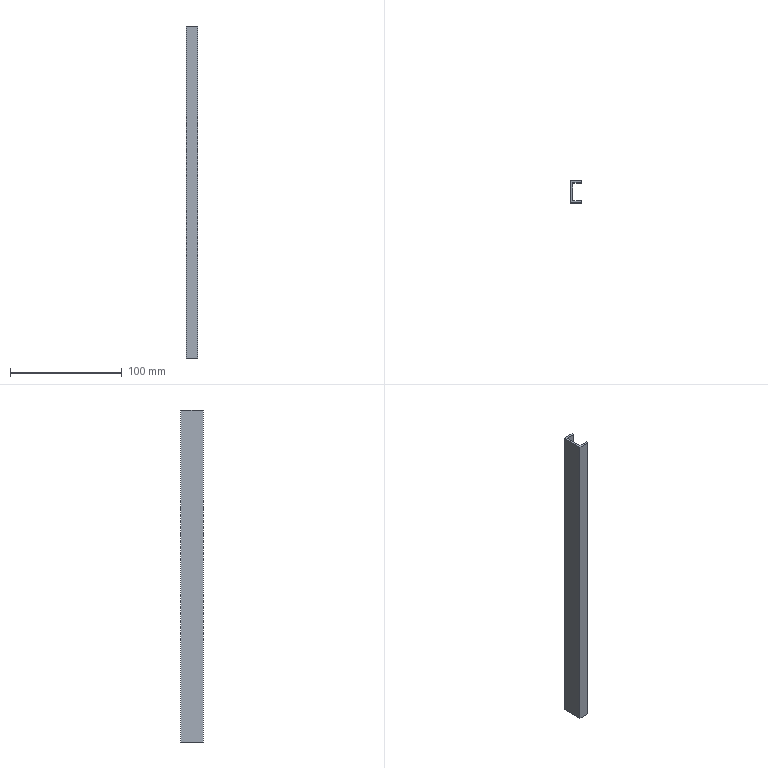Part | STEP file | 1519D1D2-4.stp.STEP | 1 solid | 10 faces | box 10 x 20 x 297 mm | volume 21384 mm3 | plane 10
STEP:
#1=CARTESIAN_POINT('',(-1.,40.,-148.5));
#2=VERTEX_POINT('',#1);
#3=CARTESIAN_POINT('',(-1.,40.,148.5));
#4=VERTEX_POINT('',#3);
#5=CARTESIAN_POINT('',(-1.,40.,-148.5));
#6=DIRECTION('',(0.,0.,1.));
#7=VECTOR('',#6,1000.);
#8=LINE('',#5,#7);
#9=EDGE_CURVE('',#2,#4,#8,.T.);
#10=ORIENTED_EDGE('',*,*,#9,.T.);
#11=CARTESIAN_POINT('',(9.,40.,148.5));
#12=VERTEX_POINT('',#11);
#13=CARTESIAN_POINT('',(-1.,40.,148.5));
#14=DIRECTION('',(1.,0.,0.));
#15=VECTOR('',#14,1000.);
#16=LINE('',#13,#15);
#17=EDGE_CURVE('',#4,#12,#16,.T.);
#18=ORIENTED_EDGE('',*,*,#17,.T.);
#19=CARTESIAN_POINT('',(9.,40.,-148.5));
#20=VERTEX_POINT('',#19);
#21=CARTESIAN_POINT('',(9.,40.,-148.5));
#22=DIRECTION('',(0.,0.,1.));
#23=VECTOR('',#22,1000.);
#24=LINE('',#21,#23);
#25=EDGE_CURVE('',#20,#12,#24,.T.);
#26=ORIENTED_EDGE('',*,*,#25,.F.);
#27=CARTESIAN_POINT('',(-1.,40.,-148.5));
#28=DIRECTION('',(1.,0.,0.));
#29=VECTOR('',#28,1000.);
#30=LINE('',#27,#29);
#31=EDGE_CURVE('',#2,#20,#30,.T.);
#32=ORIENTED_EDGE('',*,*,#31,.F.);
#33=EDGE_LOOP('',(#10,#18,#26,#32));
#34=FACE_OUTER_BOUND('',#33,.T.);
#35=CARTESIAN_POINT('',(0.,40.,0.));
#36=DIRECTION('',(0.,1.,0.));
#37=DIRECTION('',(1.,0.,0.));
#38=AXIS2_PLACEMENT_3D('',#35,#36,#37);
#39=PLANE('',#38);
#40=ADVANCED_FACE('',(#34),#39,.T.);
#41=CARTESIAN_POINT('',(1.,22.,-148.5));
#42=VERTEX_POINT('',#41);
#43=CARTESIAN_POINT('',(9.,22.,-148.5));
#44=VERTEX_POINT('',#43);
#45=CARTESIAN_POINT('',(1.,22.,-148.5));
#46=DIRECTION('',(1.,0.,0.));
#47=VECTOR('',#46,1000.);
#48=LINE('',#45,#47);
#49=EDGE_CURVE('',#42,#44,#48,.T.);
#50=ORIENTED_EDGE('',*,*,#49,.T.);
#51=CARTESIAN_POINT('',(9.,20.,-148.5));
#52=VERTEX_POINT('',#51);
#53=CARTESIAN_POINT('',(9.,20.,-148.5));
#54=DIRECTION('',(0.,1.,0.));
#55=VECTOR('',#54,1000.);
#56=LINE('',#53,#55);
#57=EDGE_CURVE('',#52,#44,#56,.T.);
#58=ORIENTED_EDGE('',*,*,#57,.F.);
#59=CARTESIAN_POINT('',(-1.,20.,-148.5));
#60=VERTEX_POINT('',#59);
#61=CARTESIAN_POINT('',(9.,20.,-148.5));
#62=DIRECTION('',(-1.,0.,0.));
#63=VECTOR('',#62,1000.);
#64=LINE('',#61,#63);
#65=EDGE_CURVE('',#52,#60,#64,.T.);
#66=ORIENTED_EDGE('',*,*,#65,.T.);
#67=CARTESIAN_POINT('',(-1.,20.,-148.5));
#68=DIRECTION('',(0.,1.,0.));
#69=VECTOR('',#68,1000.);
#70=LINE('',#67,#69);
#71=EDGE_CURVE('',#60,#2,#70,.T.);
#72=ORIENTED_EDGE('',*,*,#71,.T.);
#73=ORIENTED_EDGE('',*,*,#31,.T.);
#74=CARTESIAN_POINT('',(9.,38.,-148.5));
#75=VERTEX_POINT('',#74);
#76=CARTESIAN_POINT('',(9.,38.,-148.5));
#77=DIRECTION('',(0.,1.,0.));
#78=VECTOR('',#77,1000.);
#79=LINE('',#76,#78);
#80=EDGE_CURVE('',#75,#20,#79,.T.);
#81=ORIENTED_EDGE('',*,*,#80,.F.);
#82=CARTESIAN_POINT('',(1.,38.,-148.5));
#83=VERTEX_POINT('',#82);
#84=CARTESIAN_POINT('',(1.,38.,-148.5));
#85=DIRECTION('',(1.,0.,0.));
#86=VECTOR('',#85,1000.);
#87=LINE('',#84,#86);
#88=EDGE_CURVE('',#83,#75,#87,.T.);
#89=ORIENTED_EDGE('',*,*,#88,.F.);
#90=CARTESIAN_POINT('',(1.,22.,-148.5));
#91=DIRECTION('',(0.,1.,0.));
#92=VECTOR('',#91,1000.);
#93=LINE('',#90,#92);
#94=EDGE_CURVE('',#42,#83,#93,.T.);
#95=ORIENTED_EDGE('',*,*,#94,.F.);
#96=EDGE_LOOP('',(#50,#58,#66,#72,#73,#81,#89,#95));
#97=FACE_OUTER_BOUND('',#96,.T.);
#98=CARTESIAN_POINT('',(1.,0.,-148.5));
#99=DIRECTION('',(0.,0.,-1.));
#100=DIRECTION('',(0.,-1.,0.));
#101=AXIS2_PLACEMENT_3D('',#98,#99,#100);
#102=PLANE('',#101);
#103=ADVANCED_FACE('',(#97),#102,.T.);
#104=ORIENTED_EDGE('',*,*,#94,.T.);
#105=CARTESIAN_POINT('',(1.,38.,148.5));
#106=VERTEX_POINT('',#105);
#107=CARTESIAN_POINT('',(1.,38.,148.5));
#108=DIRECTION('',(0.,0.,-1.));
#109=VECTOR('',#108,1000.);
#110=LINE('',#107,#109);
#111=EDGE_CURVE('',#106,#83,#110,.T.);
#112=ORIENTED_EDGE('',*,*,#111,.F.);
#113=CARTESIAN_POINT('',(1.,22.,148.5));
#114=VERTEX_POINT('',#113);
#115=CARTESIAN_POINT('',(1.,22.,148.5));
#116=DIRECTION('',(0.,1.,0.));
#117=VECTOR('',#116,1000.);
#118=LINE('',#115,#117);
#119=EDGE_CURVE('',#114,#106,#118,.T.);
#120=ORIENTED_EDGE('',*,*,#119,.F.);
#121=CARTESIAN_POINT('',(1.,22.,-148.5));
#122=DIRECTION('',(0.,0.,1.));
#123=VECTOR('',#122,1000.);
#124=LINE('',#121,#123);
#125=EDGE_CURVE('',#42,#114,#124,.T.);
#126=ORIENTED_EDGE('',*,*,#125,.F.);
#127=EDGE_LOOP('',(#104,#112,#120,#126));
#128=FACE_OUTER_BOUND('',#127,.T.);
#129=CARTESIAN_POINT('',(1.,0.,148.5));
#130=DIRECTION('',(1.,0.,0.));
#131=DIRECTION('',(0.,1.,0.));
#132=AXIS2_PLACEMENT_3D('',#129,#130,#131);
#133=PLANE('',#132);
#134=ADVANCED_FACE('',(#128),#133,.T.);
#135=CARTESIAN_POINT('',(9.,22.,148.5));
#136=VERTEX_POINT('',#135);
#137=CARTESIAN_POINT('',(1.,22.,148.5));
#138=DIRECTION('',(1.,0.,0.));
#139=VECTOR('',#138,1000.);
#140=LINE('',#137,#139);
#141=EDGE_CURVE('',#114,#136,#140,.T.);
#142=ORIENTED_EDGE('',*,*,#141,.T.);
#143=CARTESIAN_POINT('',(9.,22.,-148.5));
#144=DIRECTION('',(0.,0.,1.));
#145=VECTOR('',#144,1000.);
#146=LINE('',#143,#145);
#147=EDGE_CURVE('',#44,#136,#146,.T.);
#148=ORIENTED_EDGE('',*,*,#147,.F.);
#149=ORIENTED_EDGE('',*,*,#49,.F.);
#150=ORIENTED_EDGE('',*,*,#125,.T.);
#151=EDGE_LOOP('',(#142,#148,#149,#150));
#152=FACE_OUTER_BOUND('',#151,.T.);
#153=CARTESIAN_POINT('',(1.,22.,-148.5));
#154=DIRECTION('',(0.,1.,0.));
#155=DIRECTION('',(1.,0.,0.));
#156=AXIS2_PLACEMENT_3D('',#153,#154,#155);
#157=PLANE('',#156);
#158=ADVANCED_FACE('',(#152),#157,.T.);
#159=ORIENTED_EDGE('',*,*,#147,.T.);
#160=CARTESIAN_POINT('',(9.,20.,148.5));
#161=VERTEX_POINT('',#160);
#162=CARTESIAN_POINT('',(9.,22.,148.5));
#163=DIRECTION('',(0.,-1.,0.));
#164=VECTOR('',#163,1000.);
#165=LINE('',#162,#164);
#166=EDGE_CURVE('',#136,#161,#165,.T.);
#167=ORIENTED_EDGE('',*,*,#166,.T.);
#168=CARTESIAN_POINT('',(9.,20.,148.5));
#169=DIRECTION('',(0.,0.,-1.));
#170=VECTOR('',#169,1000.);
#171=LINE('',#168,#170);
#172=EDGE_CURVE('',#161,#52,#171,.T.);
#173=ORIENTED_EDGE('',*,*,#172,.T.);
#174=ORIENTED_EDGE('',*,*,#57,.T.);
#175=EDGE_LOOP('',(#159,#167,#173,#174));
#176=FACE_OUTER_BOUND('',#175,.T.);
#177=CARTESIAN_POINT('',(9.,40.,0.));
#178=DIRECTION('',(1.,0.,0.));
#179=DIRECTION('',(0.,1.,0.));
#180=AXIS2_PLACEMENT_3D('',#177,#178,#179);
#181=PLANE('',#180);
#182=ADVANCED_FACE('',(#176),#181,.T.);
#183=CARTESIAN_POINT('',(9.,38.,148.5));
#184=VERTEX_POINT('',#183);
#185=CARTESIAN_POINT('',(9.,38.,148.5));
#186=DIRECTION('',(0.,0.,-1.));
#187=VECTOR('',#186,1000.);
#188=LINE('',#185,#187);
#189=EDGE_CURVE('',#184,#75,#188,.T.);
#190=ORIENTED_EDGE('',*,*,#189,.T.);
#191=ORIENTED_EDGE('',*,*,#80,.T.);
#192=ORIENTED_EDGE('',*,*,#25,.T.);
#193=CARTESIAN_POINT('',(9.,40.,148.5));
#194=DIRECTION('',(0.,-1.,0.));
#195=VECTOR('',#194,1000.);
#196=LINE('',#193,#195);
#197=EDGE_CURVE('',#12,#184,#196,.T.);
#198=ORIENTED_EDGE('',*,*,#197,.T.);
#199=EDGE_LOOP('',(#190,#191,#192,#198));
#200=FACE_OUTER_BOUND('',#199,.T.);
#201=CARTESIAN_POINT('',(9.,40.,0.));
#202=DIRECTION('',(1.,0.,0.));
#203=DIRECTION('',(0.,1.,0.));
#204=AXIS2_PLACEMENT_3D('',#201,#202,#203);
#205=PLANE('',#204);
#206=ADVANCED_FACE('',(#200),#205,.T.);
#207=CARTESIAN_POINT('',(-1.,20.,148.5));
#208=VERTEX_POINT('',#207);
#209=CARTESIAN_POINT('',(-1.,20.,-148.5));
#210=DIRECTION('',(0.,0.,1.));
#211=VECTOR('',#210,1000.);
#212=LINE('',#209,#211);
#213=EDGE_CURVE('',#60,#208,#212,.T.);
#214=ORIENTED_EDGE('',*,*,#213,.F.);
#215=ORIENTED_EDGE('',*,*,#65,.F.);
#216=ORIENTED_EDGE('',*,*,#172,.F.);
#217=CARTESIAN_POINT('',(9.,20.,148.5));
#218=DIRECTION('',(-1.,0.,0.));
#219=VECTOR('',#218,1000.);
#220=LINE('',#217,#219);
#221=EDGE_CURVE('',#161,#208,#220,.T.);
#222=ORIENTED_EDGE('',*,*,#221,.T.);
#223=EDGE_LOOP('',(#214,#215,#216,#222));
#224=FACE_OUTER_BOUND('',#223,.T.);
#225=CARTESIAN_POINT('',(0.,20.,0.));
#226=DIRECTION('',(0.,-1.,0.));
#227=DIRECTION('',(0.,0.,-1.));
#228=AXIS2_PLACEMENT_3D('',#225,#226,#227);
#229=PLANE('',#228);
#230=ADVANCED_FACE('',(#224),#229,.T.);
#231=CARTESIAN_POINT('',(-1.,20.,148.5));
#232=DIRECTION('',(0.,1.,0.));
#233=VECTOR('',#232,1000.);
#234=LINE('',#231,#233);
#235=EDGE_CURVE('',#208,#4,#234,.T.);
#236=ORIENTED_EDGE('',*,*,#235,.F.);
#237=ORIENTED_EDGE('',*,*,#221,.F.);
#238=ORIENTED_EDGE('',*,*,#166,.F.);
#239=ORIENTED_EDGE('',*,*,#141,.F.);
#240=ORIENTED_EDGE('',*,*,#119,.T.);
#241=CARTESIAN_POINT('',(1.,38.,148.5));
#242=DIRECTION('',(1.,0.,0.));
#243=VECTOR('',#242,1000.);
#244=LINE('',#241,#243);
#245=EDGE_CURVE('',#106,#184,#244,.T.);
#246=ORIENTED_EDGE('',*,*,#245,.T.);
#247=ORIENTED_EDGE('',*,*,#197,.F.);
#248=ORIENTED_EDGE('',*,*,#17,.F.);
#249=EDGE_LOOP('',(#236,#237,#238,#239,#240,#246,#247,#248));
#250=FACE_OUTER_BOUND('',#249,.T.);
#251=CARTESIAN_POINT('',(-1.,0.,148.5));
#252=DIRECTION('',(0.,0.,1.));
#253=DIRECTION('',(1.,0.,0.));
#254=AXIS2_PLACEMENT_3D('',#251,#252,#253);
#255=PLANE('',#254);
#256=ADVANCED_FACE('',(#250),#255,.T.);
#257=ORIENTED_EDGE('',*,*,#88,.T.);
#258=ORIENTED_EDGE('',*,*,#189,.F.);
#259=ORIENTED_EDGE('',*,*,#245,.F.);
#260=ORIENTED_EDGE('',*,*,#111,.T.);
#261=EDGE_LOOP('',(#257,#258,#259,#260));
#262=FACE_OUTER_BOUND('',#261,.T.);
#263=CARTESIAN_POINT('',(1.,38.,148.5));
#264=DIRECTION('',(0.,-1.,0.));
#265=DIRECTION('',(0.,0.,-1.));
#266=AXIS2_PLACEMENT_3D('',#263,#264,#265);
#267=PLANE('',#266);
#268=ADVANCED_FACE('',(#262),#267,.T.);
#269=ORIENTED_EDGE('',*,*,#235,.T.);
#270=ORIENTED_EDGE('',*,*,#9,.F.);
#271=ORIENTED_EDGE('',*,*,#71,.F.);
#272=ORIENTED_EDGE('',*,*,#213,.T.);
#273=EDGE_LOOP('',(#269,#270,#271,#272));
#274=FACE_OUTER_BOUND('',#273,.T.);
#275=CARTESIAN_POINT('',(-1.,0.,-148.5));
#276=DIRECTION('',(-1.,0.,0.));
#277=DIRECTION('',(0.,0.,1.));
#278=AXIS2_PLACEMENT_3D('',#275,#276,#277);
#279=PLANE('',#278);
#280=ADVANCED_FACE('',(#274),#279,.T.);
#281=CLOSED_SHELL('',(#40,#103,#134,#158,#182,#206,#230,#256,#268,#280));
#282=MANIFOLD_SOLID_BREP('',#281);
#283=CARTESIAN_POINT('',(0.,0.,0.));
#284=DIRECTION('',(0.,0.,1.));
#285=DIRECTION('',(1.,0.,0.));
#286=AXIS2_PLACEMENT_3D('',#283,#284,#285);
#287=(LENGTH_UNIT()NAMED_UNIT(*)SI_UNIT(.MILLI.,.METRE.));
#288=UNCERTAINTY_MEASURE_WITH_UNIT(LENGTH_MEASURE(0.00001),#287,'','');
#289=(NAMED_UNIT(*)PLANE_ANGLE_UNIT()SI_UNIT($,.RADIAN.));
#290=(NAMED_UNIT(*)SI_UNIT($,.STERADIAN.)SOLID_ANGLE_UNIT());
#291=(GEOMETRIC_REPRESENTATION_CONTEXT(3)GLOBAL_UNCERTAINTY_ASSIGNED_CONTEXT((#288))GLOBAL_UNIT_ASSIGNED_CONTEXT((#287,#289,#290))REPRESENTATION_CONTEXT('',''));
#292=ADVANCED_BREP_SHAPE_REPRESENTATION('',(#282,#286),#291);